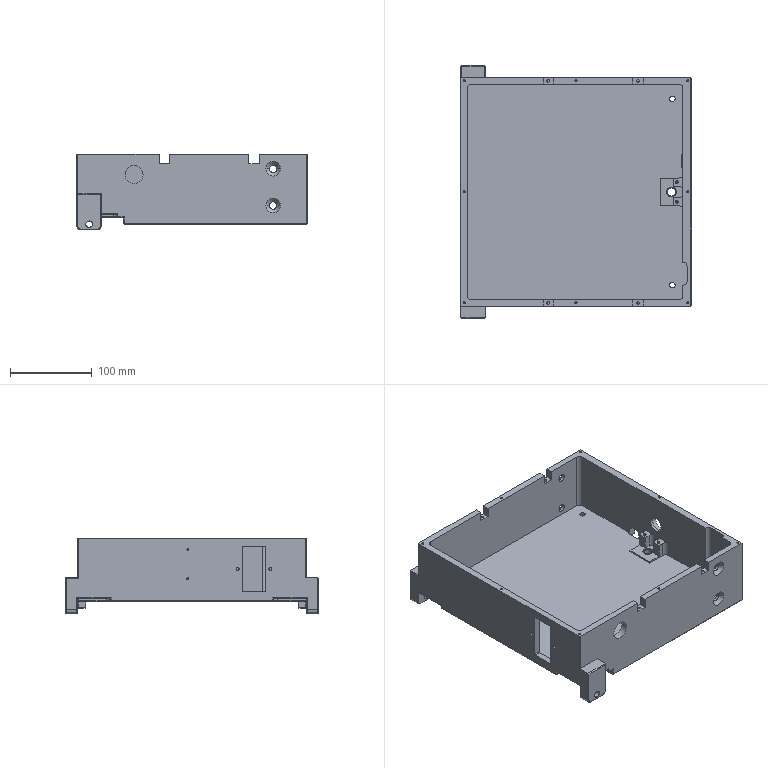Part | 1 solid | 279 faces | volume 1090125 mm3 | plane 154 | cylinder 90 | cone 34 | spline 1 | commonest cylinder face diameters 2.5 x24 10 x20 3.2 x12 9 x8 2 x4 3.5 x4